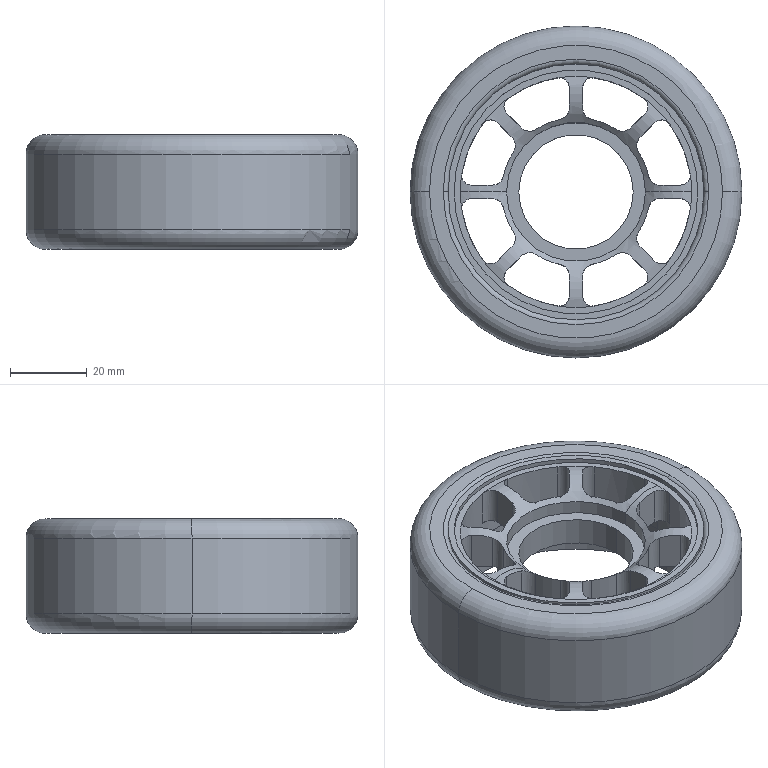Part | SolidWorks | features ICE 3, Fillet 2, Extrusion 1, Revolution 1 | 1 solid | 113 faces | box 86.769 x 86.769 x 30 mm | volume 85929 mm3 | cylinder 71 | plane 24 | torus 18 | commonest cylinder face diameters 5.08 x20 5.75 x18 41.083 x9 38.854 x8 63.744 x4 66.869 x4